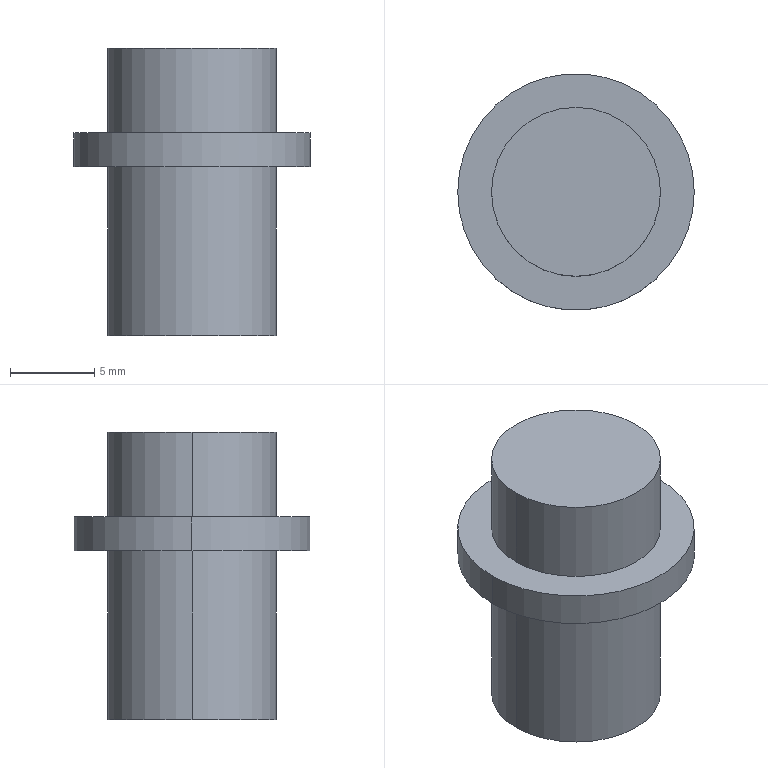Part | SolidWorks | features ICE 2, Extrusion 1 | 1 solid | 10 faces | box 14 x 14 x 17 mm | volume 1486 mm3 | cylinder 6 | plane 4 | commonest cylinder face diameters 10 x4 14 x2
STEP:
#1=CARTESIAN_POINT('',(5.,0.,17.));
#2=VERTEX_POINT('',#1);
#3=CARTESIAN_POINT('',(-5.,0.,17.));
#4=VERTEX_POINT('',#3);
#5=CARTESIAN_POINT('',(0.,0.,17.));
#6=DIRECTION('',(0.,0.,1.));
#7=DIRECTION('',(1.,0.,0.));
#8=AXIS2_PLACEMENT_3D('',#5,#6,#7);
#9=CIRCLE('',#8,5.);
#10=EDGE_CURVE('',#2,#4,#9,.T.);
#11=ORIENTED_EDGE('',*,*,#10,.F.);
#12=CARTESIAN_POINT('',(5.,0.,12.));
#13=VERTEX_POINT('',#12);
#14=CARTESIAN_POINT('',(5.,0.,17.));
#15=DIRECTION('',(0.,0.,-1.));
#16=VECTOR('',#15,1000.);
#17=LINE('',#14,#16);
#18=EDGE_CURVE('',#2,#13,#17,.T.);
#19=ORIENTED_EDGE('',*,*,#18,.T.);
#20=CARTESIAN_POINT('',(-5.,0.,12.));
#21=VERTEX_POINT('',#20);
#22=CARTESIAN_POINT('',(0.,0.,12.));
#23=DIRECTION('',(0.,0.,1.));
#24=DIRECTION('',(1.,0.,0.));
#25=AXIS2_PLACEMENT_3D('',#22,#23,#24);
#26=CIRCLE('',#25,5.);
#27=EDGE_CURVE('',#13,#21,#26,.T.);
#28=ORIENTED_EDGE('',*,*,#27,.T.);
#29=CARTESIAN_POINT('',(-5.,0.,17.));
#30=DIRECTION('',(0.,0.,-1.));
#31=VECTOR('',#30,1000.);
#32=LINE('',#29,#31);
#33=EDGE_CURVE('',#4,#21,#32,.T.);
#34=ORIENTED_EDGE('',*,*,#33,.F.);
#35=EDGE_LOOP('',(#11,#19,#28,#34));
#36=FACE_OUTER_BOUND('',#35,.T.);
#37=CARTESIAN_POINT('',(0.,0.,17.));
#38=DIRECTION('',(0.,0.,-1.));
#39=DIRECTION('',(-1.,0.,0.));
#40=AXIS2_PLACEMENT_3D('',#37,#38,#39);
#41=CYLINDRICAL_SURFACE('',#40,5.);
#42=ADVANCED_FACE('',(#36),#41,.T.);
#43=CARTESIAN_POINT('',(7.,0.,12.));
#44=VERTEX_POINT('',#43);
#45=CARTESIAN_POINT('',(-7.,0.,12.));
#46=VERTEX_POINT('',#45);
#47=CARTESIAN_POINT('',(0.,0.,12.));
#48=DIRECTION('',(0.,0.,1.));
#49=DIRECTION('',(1.,0.,0.));
#50=AXIS2_PLACEMENT_3D('',#47,#48,#49);
#51=CIRCLE('',#50,7.);
#52=EDGE_CURVE('',#44,#46,#51,.T.);
#53=ORIENTED_EDGE('',*,*,#52,.F.);
#54=CARTESIAN_POINT('',(7.,0.,10.));
#55=VERTEX_POINT('',#54);
#56=CARTESIAN_POINT('',(7.,0.,12.));
#57=DIRECTION('',(0.,0.,-1.));
#58=VECTOR('',#57,1000.);
#59=LINE('',#56,#58);
#60=EDGE_CURVE('',#44,#55,#59,.T.);
#61=ORIENTED_EDGE('',*,*,#60,.T.);
#62=CARTESIAN_POINT('',(-7.,0.,10.));
#63=VERTEX_POINT('',#62);
#64=CARTESIAN_POINT('',(0.,0.,10.));
#65=DIRECTION('',(0.,0.,1.));
#66=DIRECTION('',(1.,0.,0.));
#67=AXIS2_PLACEMENT_3D('',#64,#65,#66);
#68=CIRCLE('',#67,7.);
#69=EDGE_CURVE('',#55,#63,#68,.T.);
#70=ORIENTED_EDGE('',*,*,#69,.T.);
#71=CARTESIAN_POINT('',(-7.,0.,12.));
#72=DIRECTION('',(0.,0.,-1.));
#73=VECTOR('',#72,1000.);
#74=LINE('',#71,#73);
#75=EDGE_CURVE('',#46,#63,#74,.T.);
#76=ORIENTED_EDGE('',*,*,#75,.F.);
#77=EDGE_LOOP('',(#53,#61,#70,#76));
#78=FACE_OUTER_BOUND('',#77,.T.);
#79=CARTESIAN_POINT('',(0.,0.,12.));
#80=DIRECTION('',(0.,0.,-1.));
#81=DIRECTION('',(-1.,0.,0.));
#82=AXIS2_PLACEMENT_3D('',#79,#80,#81);
#83=CYLINDRICAL_SURFACE('',#82,7.);
#84=ADVANCED_FACE('',(#78),#83,.T.);
#85=CARTESIAN_POINT('',(5.,0.,10.));
#86=VERTEX_POINT('',#85);
#87=CARTESIAN_POINT('',(-5.,0.,10.));
#88=VERTEX_POINT('',#87);
#89=CARTESIAN_POINT('',(0.,0.,10.));
#90=DIRECTION('',(0.,0.,1.));
#91=DIRECTION('',(1.,0.,0.));
#92=AXIS2_PLACEMENT_3D('',#89,#90,#91);
#93=CIRCLE('',#92,5.);
#94=EDGE_CURVE('',#86,#88,#93,.T.);
#95=ORIENTED_EDGE('',*,*,#94,.F.);
#96=CARTESIAN_POINT('',(5.,0.,0.));
#97=VERTEX_POINT('',#96);
#98=CARTESIAN_POINT('',(5.,0.,10.));
#99=DIRECTION('',(0.,0.,-1.));
#100=VECTOR('',#99,1000.);
#101=LINE('',#98,#100);
#102=EDGE_CURVE('',#86,#97,#101,.T.);
#103=ORIENTED_EDGE('',*,*,#102,.T.);
#104=CARTESIAN_POINT('',(-5.,0.,0.));
#105=VERTEX_POINT('',#104);
#106=CARTESIAN_POINT('',(0.,0.,0.));
#107=DIRECTION('',(0.,0.,1.));
#108=DIRECTION('',(1.,0.,0.));
#109=AXIS2_PLACEMENT_3D('',#106,#107,#108);
#110=CIRCLE('',#109,5.);
#111=EDGE_CURVE('',#97,#105,#110,.T.);
#112=ORIENTED_EDGE('',*,*,#111,.T.);
#113=CARTESIAN_POINT('',(-5.,0.,10.));
#114=DIRECTION('',(0.,0.,-1.));
#115=VECTOR('',#114,1000.);
#116=LINE('',#113,#115);
#117=EDGE_CURVE('',#88,#105,#116,.T.);
#118=ORIENTED_EDGE('',*,*,#117,.F.);
#119=EDGE_LOOP('',(#95,#103,#112,#118));
#120=FACE_OUTER_BOUND('',#119,.T.);
#121=CARTESIAN_POINT('',(0.,0.,10.));
#122=DIRECTION('',(0.,0.,-1.));
#123=DIRECTION('',(-1.,0.,0.));
#124=AXIS2_PLACEMENT_3D('',#121,#122,#123);
#125=CYLINDRICAL_SURFACE('',#124,5.);
#126=ADVANCED_FACE('',(#120),#125,.T.);
#127=ORIENTED_EDGE('',*,*,#102,.F.);
#128=CARTESIAN_POINT('',(0.,0.,10.));
#129=DIRECTION('',(0.,0.,1.));
#130=DIRECTION('',(1.,0.,0.));
#131=AXIS2_PLACEMENT_3D('',#128,#129,#130);
#132=CIRCLE('',#131,5.);
#133=EDGE_CURVE('',#88,#86,#132,.T.);
#134=ORIENTED_EDGE('',*,*,#133,.F.);
#135=ORIENTED_EDGE('',*,*,#117,.T.);
#136=CARTESIAN_POINT('',(0.,0.,0.));
#137=DIRECTION('',(0.,0.,1.));
#138=DIRECTION('',(1.,0.,0.));
#139=AXIS2_PLACEMENT_3D('',#136,#137,#138);
#140=CIRCLE('',#139,5.);
#141=EDGE_CURVE('',#105,#97,#140,.T.);
#142=ORIENTED_EDGE('',*,*,#141,.T.);
#143=EDGE_LOOP('',(#127,#134,#135,#142));
#144=FACE_OUTER_BOUND('',#143,.T.);
#145=CARTESIAN_POINT('',(0.,0.,10.));
#146=DIRECTION('',(0.,0.,-1.));
#147=DIRECTION('',(-1.,0.,0.));
#148=AXIS2_PLACEMENT_3D('',#145,#146,#147);
#149=CYLINDRICAL_SURFACE('',#148,5.);
#150=ADVANCED_FACE('',(#144),#149,.T.);
#151=ORIENTED_EDGE('',*,*,#141,.F.);
#152=ORIENTED_EDGE('',*,*,#111,.F.);
#153=EDGE_LOOP('',(#151,#152));
#154=FACE_OUTER_BOUND('',#153,.T.);
#155=CARTESIAN_POINT('',(0.,0.,0.));
#156=DIRECTION('',(0.,0.,1.));
#157=DIRECTION('',(1.,0.,0.));
#158=AXIS2_PLACEMENT_3D('',#155,#156,#157);
#159=PLANE('',#158);
#160=ADVANCED_FACE('',(#154),#159,.F.);
#161=ORIENTED_EDGE('',*,*,#60,.F.);
#162=CARTESIAN_POINT('',(0.,0.,12.));
#163=DIRECTION('',(0.,0.,1.));
#164=DIRECTION('',(1.,0.,0.));
#165=AXIS2_PLACEMENT_3D('',#162,#163,#164);
#166=CIRCLE('',#165,7.);
#167=EDGE_CURVE('',#46,#44,#166,.T.);
#168=ORIENTED_EDGE('',*,*,#167,.F.);
#169=ORIENTED_EDGE('',*,*,#75,.T.);
#170=CARTESIAN_POINT('',(0.,0.,10.));
#171=DIRECTION('',(0.,0.,1.));
#172=DIRECTION('',(1.,0.,0.));
#173=AXIS2_PLACEMENT_3D('',#170,#171,#172);
#174=CIRCLE('',#173,7.);
#175=EDGE_CURVE('',#63,#55,#174,.T.);
#176=ORIENTED_EDGE('',*,*,#175,.T.);
#177=EDGE_LOOP('',(#161,#168,#169,#176));
#178=FACE_OUTER_BOUND('',#177,.T.);
#179=CARTESIAN_POINT('',(0.,0.,12.));
#180=DIRECTION('',(0.,0.,-1.));
#181=DIRECTION('',(-1.,0.,0.));
#182=AXIS2_PLACEMENT_3D('',#179,#180,#181);
#183=CYLINDRICAL_SURFACE('',#182,7.);
#184=ADVANCED_FACE('',(#178),#183,.T.);
#185=CARTESIAN_POINT('',(0.,0.,12.));
#186=DIRECTION('',(0.,0.,1.));
#187=DIRECTION('',(1.,0.,0.));
#188=AXIS2_PLACEMENT_3D('',#185,#186,#187);
#189=CIRCLE('',#188,5.);
#190=EDGE_CURVE('',#21,#13,#189,.T.);
#191=ORIENTED_EDGE('',*,*,#190,.F.);
#192=ORIENTED_EDGE('',*,*,#27,.F.);
#193=EDGE_LOOP('',(#191,#192));
#194=FACE_BOUND('',#193,.T.);
#195=ORIENTED_EDGE('',*,*,#167,.T.);
#196=ORIENTED_EDGE('',*,*,#52,.T.);
#197=EDGE_LOOP('',(#195,#196));
#198=FACE_OUTER_BOUND('',#197,.T.);
#199=CARTESIAN_POINT('',(0.,0.,12.));
#200=DIRECTION('',(0.,0.,1.));
#201=DIRECTION('',(1.,0.,0.));
#202=AXIS2_PLACEMENT_3D('',#199,#200,#201);
#203=PLANE('',#202);
#204=ADVANCED_FACE('',(#194,#198),#203,.T.);
#205=ORIENTED_EDGE('',*,*,#133,.T.);
#206=ORIENTED_EDGE('',*,*,#94,.T.);
#207=EDGE_LOOP('',(#205,#206));
#208=FACE_BOUND('',#207,.T.);
#209=ORIENTED_EDGE('',*,*,#175,.F.);
#210=ORIENTED_EDGE('',*,*,#69,.F.);
#211=EDGE_LOOP('',(#209,#210));
#212=FACE_OUTER_BOUND('',#211,.T.);
#213=CARTESIAN_POINT('',(0.,0.,10.));
#214=DIRECTION('',(0.,0.,1.));
#215=DIRECTION('',(1.,0.,0.));
#216=AXIS2_PLACEMENT_3D('',#213,#214,#215);
#217=PLANE('',#216);
#218=ADVANCED_FACE('',(#208,#212),#217,.F.);
#219=ORIENTED_EDGE('',*,*,#18,.F.);
#220=CARTESIAN_POINT('',(0.,0.,17.));
#221=DIRECTION('',(0.,0.,1.));
#222=DIRECTION('',(1.,0.,0.));
#223=AXIS2_PLACEMENT_3D('',#220,#221,#222);
#224=CIRCLE('',#223,5.);
#225=EDGE_CURVE('',#4,#2,#224,.T.);
#226=ORIENTED_EDGE('',*,*,#225,.F.);
#227=ORIENTED_EDGE('',*,*,#33,.T.);
#228=ORIENTED_EDGE('',*,*,#190,.T.);
#229=EDGE_LOOP('',(#219,#226,#227,#228));
#230=FACE_OUTER_BOUND('',#229,.T.);
#231=CARTESIAN_POINT('',(0.,0.,17.));
#232=DIRECTION('',(0.,0.,-1.));
#233=DIRECTION('',(-1.,0.,0.));
#234=AXIS2_PLACEMENT_3D('',#231,#232,#233);
#235=CYLINDRICAL_SURFACE('',#234,5.);
#236=ADVANCED_FACE('',(#230),#235,.T.);
#237=ORIENTED_EDGE('',*,*,#225,.T.);
#238=ORIENTED_EDGE('',*,*,#10,.T.);
#239=EDGE_LOOP('',(#237,#238));
#240=FACE_OUTER_BOUND('',#239,.T.);
#241=CARTESIAN_POINT('',(0.,0.,17.));
#242=DIRECTION('',(0.,0.,1.));
#243=DIRECTION('',(1.,0.,0.));
#244=AXIS2_PLACEMENT_3D('',#241,#242,#243);
#245=PLANE('',#244);
#246=ADVANCED_FACE('',(#240),#245,.T.);
#247=CLOSED_SHELL('',(#42,#84,#126,#150,#160,#184,#204,#218,#236,#246));
#248=MANIFOLD_SOLID_BREP('',#247);
#249=CARTESIAN_POINT('',(0.,0.,0.));
#250=DIRECTION('',(0.,0.,1.));
#251=DIRECTION('',(1.,0.,0.));
#252=AXIS2_PLACEMENT_3D('',#249,#250,#251);
#253=(LENGTH_UNIT()NAMED_UNIT(*)SI_UNIT(.MILLI.,.METRE.));
#254=UNCERTAINTY_MEASURE_WITH_UNIT(LENGTH_MEASURE(0.00001),#253,'','');
#255=(NAMED_UNIT(*)PLANE_ANGLE_UNIT()SI_UNIT($,.RADIAN.));
#256=(NAMED_UNIT(*)SI_UNIT($,.STERADIAN.)SOLID_ANGLE_UNIT());
#257=(GEOMETRIC_REPRESENTATION_CONTEXT(3)GLOBAL_UNCERTAINTY_ASSIGNED_CONTEXT((#254))GLOBAL_UNIT_ASSIGNED_CONTEXT((#253,#255,#256))REPRESENTATION_CONTEXT('',''));
#258=ADVANCED_BREP_SHAPE_REPRESENTATION('',(#248,#252),#257);